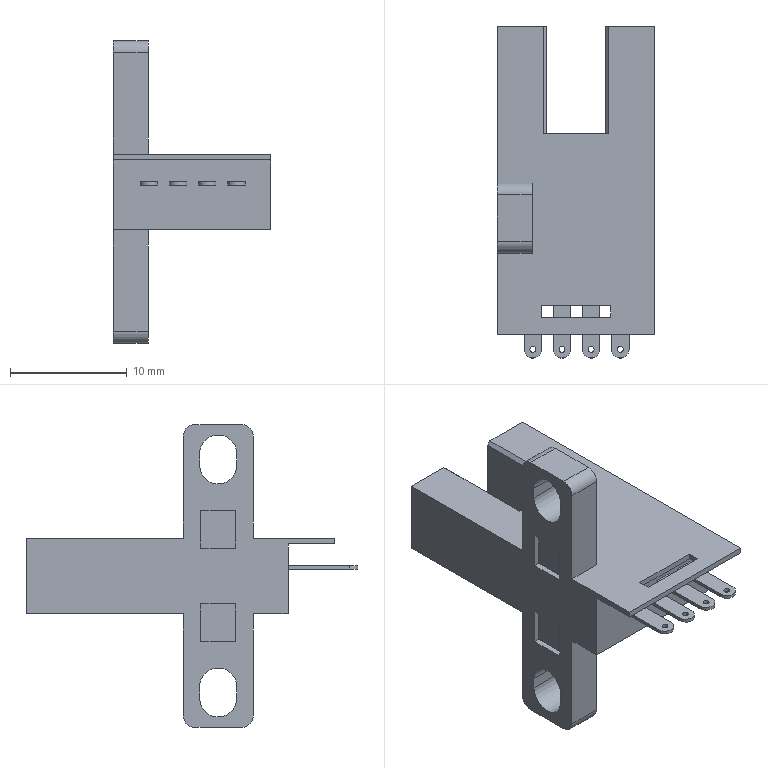Part | STEP file | EE-SX672-D12d(Omron U-shaped photoelectric) | 1 solid | 80 faces | box 13.5 x 28.5 x 26 mm | volume 1979 mm3 | plane 58 | cylinder 22 | commonest cylinder face diameters 0.5 x8 3.2 x6 1.5 x4 2 x4